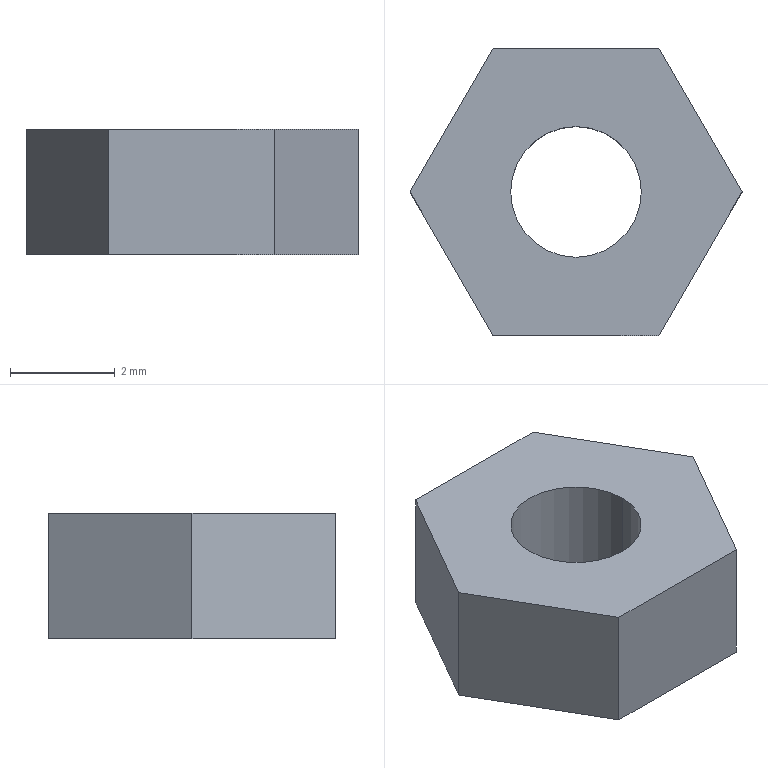Part | SolidWorks | features Extrusion 1 | 1 solid | 10 faces | box 6.351 x 5.5 x 2.4 mm | volume 51.092 mm3 | plane 8 | cylinder 2 | commonest cylinder face diameters 2.5 x2
STEP:
#1=CARTESIAN_POINT('',(-1.25,0.,-1.2));
#2=VERTEX_POINT('',#1);
#3=CARTESIAN_POINT('',(1.25,0.,-1.2));
#4=VERTEX_POINT('',#3);
#5=CARTESIAN_POINT('',(0.,0.,-1.2));
#6=DIRECTION('',(0.,0.,1.));
#7=DIRECTION('',(1.,0.,0.));
#8=AXIS2_PLACEMENT_3D('',#5,#6,#7);
#9=CIRCLE('',#8,1.25);
#10=EDGE_CURVE('',#2,#4,#9,.T.);
#11=ORIENTED_EDGE('',*,*,#10,.F.);
#12=CARTESIAN_POINT('',(-1.25,0.,1.2));
#13=VERTEX_POINT('',#12);
#14=CARTESIAN_POINT('',(-1.25,0.,-1.2));
#15=DIRECTION('',(0.,0.,1.));
#16=VECTOR('',#15,1000.);
#17=LINE('',#14,#16);
#18=EDGE_CURVE('',#2,#13,#17,.T.);
#19=ORIENTED_EDGE('',*,*,#18,.T.);
#20=CARTESIAN_POINT('',(1.25,0.,1.2));
#21=VERTEX_POINT('',#20);
#22=CARTESIAN_POINT('',(0.,0.,1.2));
#23=DIRECTION('',(0.,0.,1.));
#24=DIRECTION('',(1.,0.,0.));
#25=AXIS2_PLACEMENT_3D('',#22,#23,#24);
#26=CIRCLE('',#25,1.25);
#27=EDGE_CURVE('',#13,#21,#26,.T.);
#28=ORIENTED_EDGE('',*,*,#27,.T.);
#29=CARTESIAN_POINT('',(1.25,0.,-1.2));
#30=DIRECTION('',(0.,0.,1.));
#31=VECTOR('',#30,1000.);
#32=LINE('',#29,#31);
#33=EDGE_CURVE('',#4,#21,#32,.T.);
#34=ORIENTED_EDGE('',*,*,#33,.F.);
#35=EDGE_LOOP('',(#11,#19,#28,#34));
#36=FACE_OUTER_BOUND('',#35,.T.);
#37=CARTESIAN_POINT('',(0.,0.,-1.2));
#38=DIRECTION('',(0.,0.,1.));
#39=DIRECTION('',(1.,0.,0.));
#40=AXIS2_PLACEMENT_3D('',#37,#38,#39);
#41=CYLINDRICAL_SURFACE('',#40,1.25);
#42=ADVANCED_FACE('',(#36),#41,.F.);
#43=CARTESIAN_POINT('',(1.588,-2.75,1.2));
#44=VERTEX_POINT('',#43);
#45=CARTESIAN_POINT('',(3.175,0.,1.2));
#46=VERTEX_POINT('',#45);
#47=CARTESIAN_POINT('',(1.588,-2.75,1.2));
#48=DIRECTION('',(0.5,0.866,0.));
#49=VECTOR('',#48,1000.);
#50=LINE('',#47,#49);
#51=EDGE_CURVE('',#44,#46,#50,.T.);
#52=ORIENTED_EDGE('',*,*,#51,.F.);
#53=CARTESIAN_POINT('',(1.588,-2.75,-1.2));
#54=VERTEX_POINT('',#53);
#55=CARTESIAN_POINT('',(1.588,-2.75,-1.2));
#56=DIRECTION('',(0.,0.,1.));
#57=VECTOR('',#56,1000.);
#58=LINE('',#55,#57);
#59=EDGE_CURVE('',#54,#44,#58,.T.);
#60=ORIENTED_EDGE('',*,*,#59,.F.);
#61=CARTESIAN_POINT('',(3.175,0.,-1.2));
#62=VERTEX_POINT('',#61);
#63=CARTESIAN_POINT('',(1.588,-2.75,-1.2));
#64=DIRECTION('',(0.5,0.866,0.));
#65=VECTOR('',#64,1000.);
#66=LINE('',#63,#65);
#67=EDGE_CURVE('',#54,#62,#66,.T.);
#68=ORIENTED_EDGE('',*,*,#67,.T.);
#69=CARTESIAN_POINT('',(3.175,0.,-1.2));
#70=DIRECTION('',(0.,0.,1.));
#71=VECTOR('',#70,1000.);
#72=LINE('',#69,#71);
#73=EDGE_CURVE('',#62,#46,#72,.T.);
#74=ORIENTED_EDGE('',*,*,#73,.T.);
#75=EDGE_LOOP('',(#52,#60,#68,#74));
#76=FACE_OUTER_BOUND('',#75,.T.);
#77=CARTESIAN_POINT('',(1.588,-2.75,-1.2));
#78=DIRECTION('',(0.866,-0.5,0.));
#79=DIRECTION('',(0.5,0.866,0.));
#80=AXIS2_PLACEMENT_3D('',#77,#78,#79);
#81=PLANE('',#80);
#82=ADVANCED_FACE('',(#76),#81,.T.);
#83=CARTESIAN_POINT('',(-1.588,-2.75,1.2));
#84=VERTEX_POINT('',#83);
#85=CARTESIAN_POINT('',(-1.588,-2.75,1.2));
#86=DIRECTION('',(1.,0.,0.));
#87=VECTOR('',#86,1000.);
#88=LINE('',#85,#87);
#89=EDGE_CURVE('',#84,#44,#88,.T.);
#90=ORIENTED_EDGE('',*,*,#89,.F.);
#91=CARTESIAN_POINT('',(-1.588,-2.75,-1.2));
#92=VERTEX_POINT('',#91);
#93=CARTESIAN_POINT('',(-1.588,-2.75,-1.2));
#94=DIRECTION('',(0.,0.,1.));
#95=VECTOR('',#94,1000.);
#96=LINE('',#93,#95);
#97=EDGE_CURVE('',#92,#84,#96,.T.);
#98=ORIENTED_EDGE('',*,*,#97,.F.);
#99=CARTESIAN_POINT('',(-1.588,-2.75,-1.2));
#100=DIRECTION('',(1.,0.,0.));
#101=VECTOR('',#100,1000.);
#102=LINE('',#99,#101);
#103=EDGE_CURVE('',#92,#54,#102,.T.);
#104=ORIENTED_EDGE('',*,*,#103,.T.);
#105=ORIENTED_EDGE('',*,*,#59,.T.);
#106=EDGE_LOOP('',(#90,#98,#104,#105));
#107=FACE_OUTER_BOUND('',#106,.T.);
#108=CARTESIAN_POINT('',(-1.588,-2.75,-1.2));
#109=DIRECTION('',(0.,-1.,0.));
#110=DIRECTION('',(1.,0.,0.));
#111=AXIS2_PLACEMENT_3D('',#108,#109,#110);
#112=PLANE('',#111);
#113=ADVANCED_FACE('',(#107),#112,.T.);
#114=CARTESIAN_POINT('',(-3.175,0.,1.2));
#115=VERTEX_POINT('',#114);
#116=CARTESIAN_POINT('',(-3.175,0.,1.2));
#117=DIRECTION('',(0.5,-0.866,0.));
#118=VECTOR('',#117,1000.);
#119=LINE('',#116,#118);
#120=EDGE_CURVE('',#115,#84,#119,.T.);
#121=ORIENTED_EDGE('',*,*,#120,.F.);
#122=CARTESIAN_POINT('',(-3.175,0.,-1.2));
#123=VERTEX_POINT('',#122);
#124=CARTESIAN_POINT('',(-3.175,0.,-1.2));
#125=DIRECTION('',(0.,0.,1.));
#126=VECTOR('',#125,1000.);
#127=LINE('',#124,#126);
#128=EDGE_CURVE('',#123,#115,#127,.T.);
#129=ORIENTED_EDGE('',*,*,#128,.F.);
#130=CARTESIAN_POINT('',(-3.175,0.,-1.2));
#131=DIRECTION('',(0.5,-0.866,0.));
#132=VECTOR('',#131,1000.);
#133=LINE('',#130,#132);
#134=EDGE_CURVE('',#123,#92,#133,.T.);
#135=ORIENTED_EDGE('',*,*,#134,.T.);
#136=ORIENTED_EDGE('',*,*,#97,.T.);
#137=EDGE_LOOP('',(#121,#129,#135,#136));
#138=FACE_OUTER_BOUND('',#137,.T.);
#139=CARTESIAN_POINT('',(-3.175,0.,-1.2));
#140=DIRECTION('',(-0.866,-0.5,0.));
#141=DIRECTION('',(0.5,-0.866,0.));
#142=AXIS2_PLACEMENT_3D('',#139,#140,#141);
#143=PLANE('',#142);
#144=ADVANCED_FACE('',(#138),#143,.T.);
#145=CARTESIAN_POINT('',(-1.588,2.75,1.2));
#146=VERTEX_POINT('',#145);
#147=CARTESIAN_POINT('',(-1.588,2.75,1.2));
#148=DIRECTION('',(-0.5,-0.866,0.));
#149=VECTOR('',#148,1000.);
#150=LINE('',#147,#149);
#151=EDGE_CURVE('',#146,#115,#150,.T.);
#152=ORIENTED_EDGE('',*,*,#151,.F.);
#153=CARTESIAN_POINT('',(-1.588,2.75,-1.2));
#154=VERTEX_POINT('',#153);
#155=CARTESIAN_POINT('',(-1.588,2.75,-1.2));
#156=DIRECTION('',(0.,0.,1.));
#157=VECTOR('',#156,1000.);
#158=LINE('',#155,#157);
#159=EDGE_CURVE('',#154,#146,#158,.T.);
#160=ORIENTED_EDGE('',*,*,#159,.F.);
#161=CARTESIAN_POINT('',(-1.588,2.75,-1.2));
#162=DIRECTION('',(-0.5,-0.866,0.));
#163=VECTOR('',#162,1000.);
#164=LINE('',#161,#163);
#165=EDGE_CURVE('',#154,#123,#164,.T.);
#166=ORIENTED_EDGE('',*,*,#165,.T.);
#167=ORIENTED_EDGE('',*,*,#128,.T.);
#168=EDGE_LOOP('',(#152,#160,#166,#167));
#169=FACE_OUTER_BOUND('',#168,.T.);
#170=CARTESIAN_POINT('',(-1.588,2.75,-1.2));
#171=DIRECTION('',(-0.866,0.5,0.));
#172=DIRECTION('',(-0.5,-0.866,0.));
#173=AXIS2_PLACEMENT_3D('',#170,#171,#172);
#174=PLANE('',#173);
#175=ADVANCED_FACE('',(#169),#174,.T.);
#176=CARTESIAN_POINT('',(1.588,2.75,1.2));
#177=VERTEX_POINT('',#176);
#178=CARTESIAN_POINT('',(1.588,2.75,1.2));
#179=DIRECTION('',(-1.,0.,0.));
#180=VECTOR('',#179,1000.);
#181=LINE('',#178,#180);
#182=EDGE_CURVE('',#177,#146,#181,.T.);
#183=ORIENTED_EDGE('',*,*,#182,.F.);
#184=CARTESIAN_POINT('',(1.588,2.75,-1.2));
#185=VERTEX_POINT('',#184);
#186=CARTESIAN_POINT('',(1.588,2.75,-1.2));
#187=DIRECTION('',(0.,0.,1.));
#188=VECTOR('',#187,1000.);
#189=LINE('',#186,#188);
#190=EDGE_CURVE('',#185,#177,#189,.T.);
#191=ORIENTED_EDGE('',*,*,#190,.F.);
#192=CARTESIAN_POINT('',(1.588,2.75,-1.2));
#193=DIRECTION('',(-1.,0.,0.));
#194=VECTOR('',#193,1000.);
#195=LINE('',#192,#194);
#196=EDGE_CURVE('',#185,#154,#195,.T.);
#197=ORIENTED_EDGE('',*,*,#196,.T.);
#198=ORIENTED_EDGE('',*,*,#159,.T.);
#199=EDGE_LOOP('',(#183,#191,#197,#198));
#200=FACE_OUTER_BOUND('',#199,.T.);
#201=CARTESIAN_POINT('',(1.588,2.75,-1.2));
#202=DIRECTION('',(0.,1.,0.));
#203=DIRECTION('',(-1.,0.,0.));
#204=AXIS2_PLACEMENT_3D('',#201,#202,#203);
#205=PLANE('',#204);
#206=ADVANCED_FACE('',(#200),#205,.T.);
#207=CARTESIAN_POINT('',(3.175,0.,1.2));
#208=DIRECTION('',(-0.5,0.866,0.));
#209=VECTOR('',#208,1000.);
#210=LINE('',#207,#209);
#211=EDGE_CURVE('',#46,#177,#210,.T.);
#212=ORIENTED_EDGE('',*,*,#211,.F.);
#213=ORIENTED_EDGE('',*,*,#73,.F.);
#214=CARTESIAN_POINT('',(3.175,0.,-1.2));
#215=DIRECTION('',(-0.5,0.866,0.));
#216=VECTOR('',#215,1000.);
#217=LINE('',#214,#216);
#218=EDGE_CURVE('',#62,#185,#217,.T.);
#219=ORIENTED_EDGE('',*,*,#218,.T.);
#220=ORIENTED_EDGE('',*,*,#190,.T.);
#221=EDGE_LOOP('',(#212,#213,#219,#220));
#222=FACE_OUTER_BOUND('',#221,.T.);
#223=CARTESIAN_POINT('',(3.175,0.,-1.2));
#224=DIRECTION('',(0.866,0.5,0.));
#225=DIRECTION('',(-0.5,0.866,0.));
#226=AXIS2_PLACEMENT_3D('',#223,#224,#225);
#227=PLANE('',#226);
#228=ADVANCED_FACE('',(#222),#227,.T.);
#229=CARTESIAN_POINT('',(0.,0.,-1.2));
#230=DIRECTION('',(0.,0.,1.));
#231=DIRECTION('',(1.,0.,0.));
#232=AXIS2_PLACEMENT_3D('',#229,#230,#231);
#233=CIRCLE('',#232,1.25);
#234=EDGE_CURVE('',#4,#2,#233,.T.);
#235=ORIENTED_EDGE('',*,*,#234,.T.);
#236=ORIENTED_EDGE('',*,*,#10,.T.);
#237=EDGE_LOOP('',(#235,#236));
#238=FACE_BOUND('',#237,.T.);
#239=ORIENTED_EDGE('',*,*,#67,.F.);
#240=ORIENTED_EDGE('',*,*,#103,.F.);
#241=ORIENTED_EDGE('',*,*,#134,.F.);
#242=ORIENTED_EDGE('',*,*,#165,.F.);
#243=ORIENTED_EDGE('',*,*,#196,.F.);
#244=ORIENTED_EDGE('',*,*,#218,.F.);
#245=EDGE_LOOP('',(#239,#240,#241,#242,#243,#244));
#246=FACE_OUTER_BOUND('',#245,.T.);
#247=CARTESIAN_POINT('',(0.,0.,-1.2));
#248=DIRECTION('',(0.,0.,1.));
#249=DIRECTION('',(1.,0.,0.));
#250=AXIS2_PLACEMENT_3D('',#247,#248,#249);
#251=PLANE('',#250);
#252=ADVANCED_FACE('',(#238,#246),#251,.F.);
#253=CARTESIAN_POINT('',(0.,0.,1.2));
#254=DIRECTION('',(0.,0.,1.));
#255=DIRECTION('',(1.,0.,0.));
#256=AXIS2_PLACEMENT_3D('',#253,#254,#255);
#257=CIRCLE('',#256,1.25);
#258=EDGE_CURVE('',#21,#13,#257,.T.);
#259=ORIENTED_EDGE('',*,*,#258,.F.);
#260=ORIENTED_EDGE('',*,*,#27,.F.);
#261=EDGE_LOOP('',(#259,#260));
#262=FACE_BOUND('',#261,.T.);
#263=ORIENTED_EDGE('',*,*,#51,.T.);
#264=ORIENTED_EDGE('',*,*,#211,.T.);
#265=ORIENTED_EDGE('',*,*,#182,.T.);
#266=ORIENTED_EDGE('',*,*,#151,.T.);
#267=ORIENTED_EDGE('',*,*,#120,.T.);
#268=ORIENTED_EDGE('',*,*,#89,.T.);
#269=EDGE_LOOP('',(#263,#264,#265,#266,#267,#268));
#270=FACE_OUTER_BOUND('',#269,.T.);
#271=CARTESIAN_POINT('',(0.,0.,1.2));
#272=DIRECTION('',(0.,0.,1.));
#273=DIRECTION('',(1.,0.,0.));
#274=AXIS2_PLACEMENT_3D('',#271,#272,#273);
#275=PLANE('',#274);
#276=ADVANCED_FACE('',(#262,#270),#275,.T.);
#277=ORIENTED_EDGE('',*,*,#18,.F.);
#278=ORIENTED_EDGE('',*,*,#234,.F.);
#279=ORIENTED_EDGE('',*,*,#33,.T.);
#280=ORIENTED_EDGE('',*,*,#258,.T.);
#281=EDGE_LOOP('',(#277,#278,#279,#280));
#282=FACE_OUTER_BOUND('',#281,.T.);
#283=CARTESIAN_POINT('',(0.,0.,-1.2));
#284=DIRECTION('',(0.,0.,1.));
#285=DIRECTION('',(1.,0.,0.));
#286=AXIS2_PLACEMENT_3D('',#283,#284,#285);
#287=CYLINDRICAL_SURFACE('',#286,1.25);
#288=ADVANCED_FACE('',(#282),#287,.F.);
#289=CLOSED_SHELL('',(#42,#82,#113,#144,#175,#206,#228,#252,#276,#288));
#290=MANIFOLD_SOLID_BREP('',#289);
#291=CARTESIAN_POINT('',(0.,0.,0.));
#292=DIRECTION('',(0.,0.,1.));
#293=DIRECTION('',(1.,0.,0.));
#294=AXIS2_PLACEMENT_3D('',#291,#292,#293);
#295=(LENGTH_UNIT()NAMED_UNIT(*)SI_UNIT(.MILLI.,.METRE.));
#296=UNCERTAINTY_MEASURE_WITH_UNIT(LENGTH_MEASURE(0.00001),#295,'','');
#297=(NAMED_UNIT(*)PLANE_ANGLE_UNIT()SI_UNIT($,.RADIAN.));
#298=(NAMED_UNIT(*)SI_UNIT($,.STERADIAN.)SOLID_ANGLE_UNIT());
#299=(GEOMETRIC_REPRESENTATION_CONTEXT(3)GLOBAL_UNCERTAINTY_ASSIGNED_CONTEXT((#296))GLOBAL_UNIT_ASSIGNED_CONTEXT((#295,#297,#298))REPRESENTATION_CONTEXT('',''));
#300=ADVANCED_BREP_SHAPE_REPRESENTATION('',(#290,#294),#299);